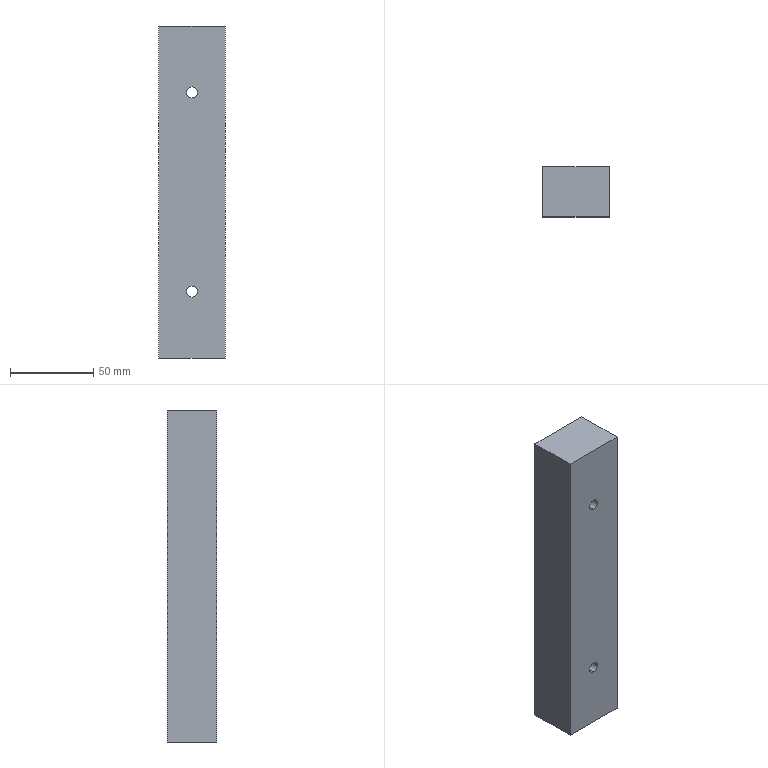Part | SolidWorks | features Extrusion 1, HoleWzd 1 | 1 solid | 16 faces | box 40 x 30 x 200 mm | volume 236731 mm3 | cylinder 8 | plane 8 | commonest cylinder face diameters 6.6 x4 11 x4
STEP:
#1=CARTESIAN_POINT('',(0.,5.,-65.5));
#2=VERTEX_POINT('',#1);
#3=CARTESIAN_POINT('',(0.,5.,-54.5));
#4=VERTEX_POINT('',#3);
#5=CARTESIAN_POINT('',(0.,5.,-60.));
#6=DIRECTION('',(0.,1.,0.));
#7=DIRECTION('',(0.,0.,1.));
#8=AXIS2_PLACEMENT_3D('',#5,#6,#7);
#9=CIRCLE('',#8,5.5);
#10=EDGE_CURVE('',#2,#4,#9,.T.);
#11=ORIENTED_EDGE('',*,*,#10,.F.);
#12=CARTESIAN_POINT('',(0.,15.,-65.5));
#13=VERTEX_POINT('',#12);
#14=CARTESIAN_POINT('',(0.,15.,-65.5));
#15=DIRECTION('',(0.,1.,0.));
#16=VECTOR('',#15,1000.);
#17=LINE('',#14,#16);
#18=EDGE_CURVE('',#2,#13,#17,.T.);
#19=ORIENTED_EDGE('',*,*,#18,.T.);
#20=CARTESIAN_POINT('',(0.,15.,-54.5));
#21=VERTEX_POINT('',#20);
#22=CARTESIAN_POINT('',(0.,15.,-60.));
#23=DIRECTION('',(0.,1.,0.));
#24=DIRECTION('',(0.,0.,1.));
#25=AXIS2_PLACEMENT_3D('',#22,#23,#24);
#26=CIRCLE('',#25,5.5);
#27=EDGE_CURVE('',#13,#21,#26,.T.);
#28=ORIENTED_EDGE('',*,*,#27,.T.);
#29=CARTESIAN_POINT('',(0.,15.,-54.5));
#30=DIRECTION('',(0.,1.,0.));
#31=VECTOR('',#30,1000.);
#32=LINE('',#29,#31);
#33=EDGE_CURVE('',#4,#21,#32,.T.);
#34=ORIENTED_EDGE('',*,*,#33,.F.);
#35=EDGE_LOOP('',(#11,#19,#28,#34));
#36=FACE_OUTER_BOUND('',#35,.T.);
#37=CARTESIAN_POINT('',(0.,15.,-60.));
#38=DIRECTION('',(0.,1.,0.));
#39=DIRECTION('',(0.,0.,1.));
#40=AXIS2_PLACEMENT_3D('',#37,#38,#39);
#41=CYLINDRICAL_SURFACE('',#40,5.5);
#42=ADVANCED_FACE('',(#36),#41,.F.);
#43=CARTESIAN_POINT('',(0.,-15.,-63.3));
#44=VERTEX_POINT('',#43);
#45=CARTESIAN_POINT('',(0.,-15.,-56.7));
#46=VERTEX_POINT('',#45);
#47=CARTESIAN_POINT('',(0.,-15.,-60.));
#48=DIRECTION('',(0.,1.,0.));
#49=DIRECTION('',(0.,0.,1.));
#50=AXIS2_PLACEMENT_3D('',#47,#48,#49);
#51=CIRCLE('',#50,3.3);
#52=EDGE_CURVE('',#44,#46,#51,.T.);
#53=ORIENTED_EDGE('',*,*,#52,.F.);
#54=CARTESIAN_POINT('',(0.,5.,-63.3));
#55=VERTEX_POINT('',#54);
#56=CARTESIAN_POINT('',(0.,15.,-63.3));
#57=DIRECTION('',(0.,1.,0.));
#58=VECTOR('',#57,1000.);
#59=LINE('',#56,#58);
#60=EDGE_CURVE('',#44,#55,#59,.T.);
#61=ORIENTED_EDGE('',*,*,#60,.T.);
#62=CARTESIAN_POINT('',(0.,5.,-56.7));
#63=VERTEX_POINT('',#62);
#64=CARTESIAN_POINT('',(0.,5.,-60.));
#65=DIRECTION('',(0.,1.,0.));
#66=DIRECTION('',(0.,0.,1.));
#67=AXIS2_PLACEMENT_3D('',#64,#65,#66);
#68=CIRCLE('',#67,3.3);
#69=EDGE_CURVE('',#55,#63,#68,.T.);
#70=ORIENTED_EDGE('',*,*,#69,.T.);
#71=CARTESIAN_POINT('',(0.,15.,-56.7));
#72=DIRECTION('',(0.,1.,0.));
#73=VECTOR('',#72,1000.);
#74=LINE('',#71,#73);
#75=EDGE_CURVE('',#46,#63,#74,.T.);
#76=ORIENTED_EDGE('',*,*,#75,.F.);
#77=EDGE_LOOP('',(#53,#61,#70,#76));
#78=FACE_OUTER_BOUND('',#77,.T.);
#79=CARTESIAN_POINT('',(0.,15.,-60.));
#80=DIRECTION('',(0.,1.,0.));
#81=DIRECTION('',(0.,0.,1.));
#82=AXIS2_PLACEMENT_3D('',#79,#80,#81);
#83=CYLINDRICAL_SURFACE('',#82,3.3);
#84=ADVANCED_FACE('',(#78),#83,.F.);
#85=CARTESIAN_POINT('',(0.,5.,54.5));
#86=VERTEX_POINT('',#85);
#87=CARTESIAN_POINT('',(0.,5.,65.5));
#88=VERTEX_POINT('',#87);
#89=CARTESIAN_POINT('',(0.,5.,60.));
#90=DIRECTION('',(0.,1.,0.));
#91=DIRECTION('',(0.,0.,1.));
#92=AXIS2_PLACEMENT_3D('',#89,#90,#91);
#93=CIRCLE('',#92,5.5);
#94=EDGE_CURVE('',#86,#88,#93,.T.);
#95=ORIENTED_EDGE('',*,*,#94,.F.);
#96=CARTESIAN_POINT('',(0.,15.,54.5));
#97=VERTEX_POINT('',#96);
#98=CARTESIAN_POINT('',(0.,15.,54.5));
#99=DIRECTION('',(0.,1.,0.));
#100=VECTOR('',#99,1000.);
#101=LINE('',#98,#100);
#102=EDGE_CURVE('',#86,#97,#101,.T.);
#103=ORIENTED_EDGE('',*,*,#102,.T.);
#104=CARTESIAN_POINT('',(0.,15.,65.5));
#105=VERTEX_POINT('',#104);
#106=CARTESIAN_POINT('',(0.,15.,60.));
#107=DIRECTION('',(0.,1.,0.));
#108=DIRECTION('',(0.,0.,1.));
#109=AXIS2_PLACEMENT_3D('',#106,#107,#108);
#110=CIRCLE('',#109,5.5);
#111=EDGE_CURVE('',#97,#105,#110,.T.);
#112=ORIENTED_EDGE('',*,*,#111,.T.);
#113=CARTESIAN_POINT('',(0.,15.,65.5));
#114=DIRECTION('',(0.,1.,0.));
#115=VECTOR('',#114,1000.);
#116=LINE('',#113,#115);
#117=EDGE_CURVE('',#88,#105,#116,.T.);
#118=ORIENTED_EDGE('',*,*,#117,.F.);
#119=EDGE_LOOP('',(#95,#103,#112,#118));
#120=FACE_OUTER_BOUND('',#119,.T.);
#121=CARTESIAN_POINT('',(0.,15.,60.));
#122=DIRECTION('',(0.,1.,0.));
#123=DIRECTION('',(0.,0.,1.));
#124=AXIS2_PLACEMENT_3D('',#121,#122,#123);
#125=CYLINDRICAL_SURFACE('',#124,5.5);
#126=ADVANCED_FACE('',(#120),#125,.F.);
#127=CARTESIAN_POINT('',(0.,-15.,56.7));
#128=VERTEX_POINT('',#127);
#129=CARTESIAN_POINT('',(0.,-15.,63.3));
#130=VERTEX_POINT('',#129);
#131=CARTESIAN_POINT('',(0.,-15.,60.));
#132=DIRECTION('',(0.,1.,0.));
#133=DIRECTION('',(0.,0.,1.));
#134=AXIS2_PLACEMENT_3D('',#131,#132,#133);
#135=CIRCLE('',#134,3.3);
#136=EDGE_CURVE('',#128,#130,#135,.T.);
#137=ORIENTED_EDGE('',*,*,#136,.F.);
#138=CARTESIAN_POINT('',(0.,5.,56.7));
#139=VERTEX_POINT('',#138);
#140=CARTESIAN_POINT('',(0.,15.,56.7));
#141=DIRECTION('',(0.,1.,0.));
#142=VECTOR('',#141,1000.);
#143=LINE('',#140,#142);
#144=EDGE_CURVE('',#128,#139,#143,.T.);
#145=ORIENTED_EDGE('',*,*,#144,.T.);
#146=CARTESIAN_POINT('',(0.,5.,63.3));
#147=VERTEX_POINT('',#146);
#148=CARTESIAN_POINT('',(0.,5.,60.));
#149=DIRECTION('',(0.,1.,0.));
#150=DIRECTION('',(0.,0.,1.));
#151=AXIS2_PLACEMENT_3D('',#148,#149,#150);
#152=CIRCLE('',#151,3.3);
#153=EDGE_CURVE('',#139,#147,#152,.T.);
#154=ORIENTED_EDGE('',*,*,#153,.T.);
#155=CARTESIAN_POINT('',(0.,15.,63.3));
#156=DIRECTION('',(0.,1.,0.));
#157=VECTOR('',#156,1000.);
#158=LINE('',#155,#157);
#159=EDGE_CURVE('',#130,#147,#158,.T.);
#160=ORIENTED_EDGE('',*,*,#159,.F.);
#161=EDGE_LOOP('',(#137,#145,#154,#160));
#162=FACE_OUTER_BOUND('',#161,.T.);
#163=CARTESIAN_POINT('',(0.,15.,60.));
#164=DIRECTION('',(0.,1.,0.));
#165=DIRECTION('',(0.,0.,1.));
#166=AXIS2_PLACEMENT_3D('',#163,#164,#165);
#167=CYLINDRICAL_SURFACE('',#166,3.3);
#168=ADVANCED_FACE('',(#162),#167,.F.);
#169=CARTESIAN_POINT('',(20.,-15.,100.));
#170=VERTEX_POINT('',#169);
#171=CARTESIAN_POINT('',(20.,-15.,-100.));
#172=VERTEX_POINT('',#171);
#173=CARTESIAN_POINT('',(20.,-15.,100.));
#174=DIRECTION('',(0.,0.,-1.));
#175=VECTOR('',#174,1000.);
#176=LINE('',#173,#175);
#177=EDGE_CURVE('',#170,#172,#176,.T.);
#178=ORIENTED_EDGE('',*,*,#177,.T.);
#179=CARTESIAN_POINT('',(20.,15.,-100.));
#180=VERTEX_POINT('',#179);
#181=CARTESIAN_POINT('',(20.,15.,-100.));
#182=DIRECTION('',(0.,-1.,0.));
#183=VECTOR('',#182,1000.);
#184=LINE('',#181,#183);
#185=EDGE_CURVE('',#180,#172,#184,.T.);
#186=ORIENTED_EDGE('',*,*,#185,.F.);
#187=CARTESIAN_POINT('',(20.,15.,100.));
#188=VERTEX_POINT('',#187);
#189=CARTESIAN_POINT('',(20.,15.,100.));
#190=DIRECTION('',(0.,0.,-1.));
#191=VECTOR('',#190,1000.);
#192=LINE('',#189,#191);
#193=EDGE_CURVE('',#188,#180,#192,.T.);
#194=ORIENTED_EDGE('',*,*,#193,.F.);
#195=CARTESIAN_POINT('',(20.,15.,100.));
#196=DIRECTION('',(0.,-1.,0.));
#197=VECTOR('',#196,1000.);
#198=LINE('',#195,#197);
#199=EDGE_CURVE('',#188,#170,#198,.T.);
#200=ORIENTED_EDGE('',*,*,#199,.T.);
#201=EDGE_LOOP('',(#178,#186,#194,#200));
#202=FACE_OUTER_BOUND('',#201,.T.);
#203=CARTESIAN_POINT('',(20.,15.,100.));
#204=DIRECTION('',(-1.,0.,0.));
#205=DIRECTION('',(0.,0.,1.));
#206=AXIS2_PLACEMENT_3D('',#203,#204,#205);
#207=PLANE('',#206);
#208=ADVANCED_FACE('',(#202),#207,.F.);
#209=CARTESIAN_POINT('',(-20.,-15.,-100.));
#210=VERTEX_POINT('',#209);
#211=CARTESIAN_POINT('',(-20.,-15.,-100.));
#212=DIRECTION('',(-1.,0.,0.));
#213=VECTOR('',#212,1000.);
#214=LINE('',#211,#213);
#215=EDGE_CURVE('',#172,#210,#214,.T.);
#216=ORIENTED_EDGE('',*,*,#215,.T.);
#217=CARTESIAN_POINT('',(-20.,15.,-100.));
#218=VERTEX_POINT('',#217);
#219=CARTESIAN_POINT('',(-20.,15.,-100.));
#220=DIRECTION('',(0.,-1.,0.));
#221=VECTOR('',#220,1000.);
#222=LINE('',#219,#221);
#223=EDGE_CURVE('',#218,#210,#222,.T.);
#224=ORIENTED_EDGE('',*,*,#223,.F.);
#225=CARTESIAN_POINT('',(-20.,15.,-100.));
#226=DIRECTION('',(-1.,0.,0.));
#227=VECTOR('',#226,1000.);
#228=LINE('',#225,#227);
#229=EDGE_CURVE('',#180,#218,#228,.T.);
#230=ORIENTED_EDGE('',*,*,#229,.F.);
#231=ORIENTED_EDGE('',*,*,#185,.T.);
#232=EDGE_LOOP('',(#216,#224,#230,#231));
#233=FACE_OUTER_BOUND('',#232,.T.);
#234=CARTESIAN_POINT('',(-20.,15.,-100.));
#235=DIRECTION('',(0.,0.,1.));
#236=DIRECTION('',(1.,0.,0.));
#237=AXIS2_PLACEMENT_3D('',#234,#235,#236);
#238=PLANE('',#237);
#239=ADVANCED_FACE('',(#233),#238,.F.);
#240=CARTESIAN_POINT('',(-20.,-15.,100.));
#241=VERTEX_POINT('',#240);
#242=CARTESIAN_POINT('',(-20.,-15.,100.));
#243=DIRECTION('',(0.,0.,1.));
#244=VECTOR('',#243,1000.);
#245=LINE('',#242,#244);
#246=EDGE_CURVE('',#210,#241,#245,.T.);
#247=ORIENTED_EDGE('',*,*,#246,.T.);
#248=CARTESIAN_POINT('',(-20.,15.,100.));
#249=VERTEX_POINT('',#248);
#250=CARTESIAN_POINT('',(-20.,15.,100.));
#251=DIRECTION('',(0.,-1.,0.));
#252=VECTOR('',#251,1000.);
#253=LINE('',#250,#252);
#254=EDGE_CURVE('',#249,#241,#253,.T.);
#255=ORIENTED_EDGE('',*,*,#254,.F.);
#256=CARTESIAN_POINT('',(-20.,15.,100.));
#257=DIRECTION('',(0.,0.,1.));
#258=VECTOR('',#257,1000.);
#259=LINE('',#256,#258);
#260=EDGE_CURVE('',#218,#249,#259,.T.);
#261=ORIENTED_EDGE('',*,*,#260,.F.);
#262=ORIENTED_EDGE('',*,*,#223,.T.);
#263=EDGE_LOOP('',(#247,#255,#261,#262));
#264=FACE_OUTER_BOUND('',#263,.T.);
#265=CARTESIAN_POINT('',(-20.,15.,100.));
#266=DIRECTION('',(1.,0.,0.));
#267=DIRECTION('',(0.,0.,-1.));
#268=AXIS2_PLACEMENT_3D('',#265,#266,#267);
#269=PLANE('',#268);
#270=ADVANCED_FACE('',(#264),#269,.F.);
#271=CARTESIAN_POINT('',(-20.,-15.,100.));
#272=DIRECTION('',(1.,0.,0.));
#273=VECTOR('',#272,1000.);
#274=LINE('',#271,#273);
#275=EDGE_CURVE('',#241,#170,#274,.T.);
#276=ORIENTED_EDGE('',*,*,#275,.T.);
#277=ORIENTED_EDGE('',*,*,#199,.F.);
#278=CARTESIAN_POINT('',(-20.,15.,100.));
#279=DIRECTION('',(1.,0.,0.));
#280=VECTOR('',#279,1000.);
#281=LINE('',#278,#280);
#282=EDGE_CURVE('',#249,#188,#281,.T.);
#283=ORIENTED_EDGE('',*,*,#282,.F.);
#284=ORIENTED_EDGE('',*,*,#254,.T.);
#285=EDGE_LOOP('',(#276,#277,#283,#284));
#286=FACE_OUTER_BOUND('',#285,.T.);
#287=CARTESIAN_POINT('',(-20.,15.,100.));
#288=DIRECTION('',(0.,0.,-1.));
#289=DIRECTION('',(-1.,0.,0.));
#290=AXIS2_PLACEMENT_3D('',#287,#288,#289);
#291=PLANE('',#290);
#292=ADVANCED_FACE('',(#286),#291,.F.);
#293=CARTESIAN_POINT('',(0.,15.,-60.));
#294=DIRECTION('',(0.,1.,0.));
#295=DIRECTION('',(0.,0.,1.));
#296=AXIS2_PLACEMENT_3D('',#293,#294,#295);
#297=CIRCLE('',#296,5.5);
#298=EDGE_CURVE('',#21,#13,#297,.T.);
#299=ORIENTED_EDGE('',*,*,#298,.F.);
#300=ORIENTED_EDGE('',*,*,#27,.F.);
#301=EDGE_LOOP('',(#299,#300));
#302=FACE_BOUND('',#301,.T.);
#303=CARTESIAN_POINT('',(0.,15.,60.));
#304=DIRECTION('',(0.,1.,0.));
#305=DIRECTION('',(0.,0.,1.));
#306=AXIS2_PLACEMENT_3D('',#303,#304,#305);
#307=CIRCLE('',#306,5.5);
#308=EDGE_CURVE('',#105,#97,#307,.T.);
#309=ORIENTED_EDGE('',*,*,#308,.F.);
#310=ORIENTED_EDGE('',*,*,#111,.F.);
#311=EDGE_LOOP('',(#309,#310));
#312=FACE_BOUND('',#311,.T.);
#313=ORIENTED_EDGE('',*,*,#193,.T.);
#314=ORIENTED_EDGE('',*,*,#229,.T.);
#315=ORIENTED_EDGE('',*,*,#260,.T.);
#316=ORIENTED_EDGE('',*,*,#282,.T.);
#317=EDGE_LOOP('',(#313,#314,#315,#316));
#318=FACE_OUTER_BOUND('',#317,.T.);
#319=CARTESIAN_POINT('',(0.,15.,0.));
#320=DIRECTION('',(0.,-1.,0.));
#321=DIRECTION('',(0.,0.,-1.));
#322=AXIS2_PLACEMENT_3D('',#319,#320,#321);
#323=PLANE('',#322);
#324=ADVANCED_FACE('',(#302,#312,#318),#323,.F.);
#325=CARTESIAN_POINT('',(0.,-15.,-60.));
#326=DIRECTION('',(0.,1.,0.));
#327=DIRECTION('',(0.,0.,1.));
#328=AXIS2_PLACEMENT_3D('',#325,#326,#327);
#329=CIRCLE('',#328,3.3);
#330=EDGE_CURVE('',#46,#44,#329,.T.);
#331=ORIENTED_EDGE('',*,*,#330,.T.);
#332=ORIENTED_EDGE('',*,*,#52,.T.);
#333=EDGE_LOOP('',(#331,#332));
#334=FACE_BOUND('',#333,.T.);
#335=CARTESIAN_POINT('',(0.,-15.,60.));
#336=DIRECTION('',(0.,1.,0.));
#337=DIRECTION('',(0.,0.,1.));
#338=AXIS2_PLACEMENT_3D('',#335,#336,#337);
#339=CIRCLE('',#338,3.3);
#340=EDGE_CURVE('',#130,#128,#339,.T.);
#341=ORIENTED_EDGE('',*,*,#340,.T.);
#342=ORIENTED_EDGE('',*,*,#136,.T.);
#343=EDGE_LOOP('',(#341,#342));
#344=FACE_BOUND('',#343,.T.);
#345=ORIENTED_EDGE('',*,*,#177,.F.);
#346=ORIENTED_EDGE('',*,*,#275,.F.);
#347=ORIENTED_EDGE('',*,*,#246,.F.);
#348=ORIENTED_EDGE('',*,*,#215,.F.);
#349=EDGE_LOOP('',(#345,#346,#347,#348));
#350=FACE_OUTER_BOUND('',#349,.T.);
#351=CARTESIAN_POINT('',(0.,-15.,0.));
#352=DIRECTION('',(0.,-1.,0.));
#353=DIRECTION('',(0.,0.,-1.));
#354=AXIS2_PLACEMENT_3D('',#351,#352,#353);
#355=PLANE('',#354);
#356=ADVANCED_FACE('',(#334,#344,#350),#355,.T.);
#357=ORIENTED_EDGE('',*,*,#144,.F.);
#358=ORIENTED_EDGE('',*,*,#340,.F.);
#359=ORIENTED_EDGE('',*,*,#159,.T.);
#360=CARTESIAN_POINT('',(0.,5.,60.));
#361=DIRECTION('',(0.,1.,0.));
#362=DIRECTION('',(0.,0.,1.));
#363=AXIS2_PLACEMENT_3D('',#360,#361,#362);
#364=CIRCLE('',#363,3.3);
#365=EDGE_CURVE('',#147,#139,#364,.T.);
#366=ORIENTED_EDGE('',*,*,#365,.T.);
#367=EDGE_LOOP('',(#357,#358,#359,#366));
#368=FACE_OUTER_BOUND('',#367,.T.);
#369=CARTESIAN_POINT('',(0.,15.,60.));
#370=DIRECTION('',(0.,1.,0.));
#371=DIRECTION('',(0.,0.,1.));
#372=AXIS2_PLACEMENT_3D('',#369,#370,#371);
#373=CYLINDRICAL_SURFACE('',#372,3.3);
#374=ADVANCED_FACE('',(#368),#373,.F.);
#375=ORIENTED_EDGE('',*,*,#365,.F.);
#376=ORIENTED_EDGE('',*,*,#153,.F.);
#377=EDGE_LOOP('',(#375,#376));
#378=FACE_BOUND('',#377,.T.);
#379=CARTESIAN_POINT('',(0.,5.,60.));
#380=DIRECTION('',(0.,1.,0.));
#381=DIRECTION('',(0.,0.,1.));
#382=AXIS2_PLACEMENT_3D('',#379,#380,#381);
#383=CIRCLE('',#382,5.5);
#384=EDGE_CURVE('',#88,#86,#383,.T.);
#385=ORIENTED_EDGE('',*,*,#384,.T.);
#386=ORIENTED_EDGE('',*,*,#94,.T.);
#387=EDGE_LOOP('',(#385,#386));
#388=FACE_OUTER_BOUND('',#387,.T.);
#389=CARTESIAN_POINT('',(3.3,5.,60.));
#390=DIRECTION('',(0.,-1.,0.));
#391=DIRECTION('',(0.,0.,-1.));
#392=AXIS2_PLACEMENT_3D('',#389,#390,#391);
#393=PLANE('',#392);
#394=ADVANCED_FACE('',(#378,#388),#393,.F.);
#395=ORIENTED_EDGE('',*,*,#102,.F.);
#396=ORIENTED_EDGE('',*,*,#384,.F.);
#397=ORIENTED_EDGE('',*,*,#117,.T.);
#398=ORIENTED_EDGE('',*,*,#308,.T.);
#399=EDGE_LOOP('',(#395,#396,#397,#398));
#400=FACE_OUTER_BOUND('',#399,.T.);
#401=CARTESIAN_POINT('',(0.,15.,60.));
#402=DIRECTION('',(0.,1.,0.));
#403=DIRECTION('',(0.,0.,1.));
#404=AXIS2_PLACEMENT_3D('',#401,#402,#403);
#405=CYLINDRICAL_SURFACE('',#404,5.5);
#406=ADVANCED_FACE('',(#400),#405,.F.);
#407=ORIENTED_EDGE('',*,*,#60,.F.);
#408=ORIENTED_EDGE('',*,*,#330,.F.);
#409=ORIENTED_EDGE('',*,*,#75,.T.);
#410=CARTESIAN_POINT('',(0.,5.,-60.));
#411=DIRECTION('',(0.,1.,0.));
#412=DIRECTION('',(0.,0.,1.));
#413=AXIS2_PLACEMENT_3D('',#410,#411,#412);
#414=CIRCLE('',#413,3.3);
#415=EDGE_CURVE('',#63,#55,#414,.T.);
#416=ORIENTED_EDGE('',*,*,#415,.T.);
#417=EDGE_LOOP('',(#407,#408,#409,#416));
#418=FACE_OUTER_BOUND('',#417,.T.);
#419=CARTESIAN_POINT('',(0.,15.,-60.));
#420=DIRECTION('',(0.,1.,0.));
#421=DIRECTION('',(0.,0.,1.));
#422=AXIS2_PLACEMENT_3D('',#419,#420,#421);
#423=CYLINDRICAL_SURFACE('',#422,3.3);
#424=ADVANCED_FACE('',(#418),#423,.F.);
#425=ORIENTED_EDGE('',*,*,#415,.F.);
#426=ORIENTED_EDGE('',*,*,#69,.F.);
#427=EDGE_LOOP('',(#425,#426));
#428=FACE_BOUND('',#427,.T.);
#429=CARTESIAN_POINT('',(0.,5.,-60.));
#430=DIRECTION('',(0.,1.,0.));
#431=DIRECTION('',(0.,0.,1.));
#432=AXIS2_PLACEMENT_3D('',#429,#430,#431);
#433=CIRCLE('',#432,5.5);
#434=EDGE_CURVE('',#4,#2,#433,.T.);
#435=ORIENTED_EDGE('',*,*,#434,.T.);
#436=ORIENTED_EDGE('',*,*,#10,.T.);
#437=EDGE_LOOP('',(#435,#436));
#438=FACE_OUTER_BOUND('',#437,.T.);
#439=CARTESIAN_POINT('',(3.3,5.,-60.));
#440=DIRECTION('',(0.,-1.,0.));
#441=DIRECTION('',(0.,0.,-1.));
#442=AXIS2_PLACEMENT_3D('',#439,#440,#441);
#443=PLANE('',#442);
#444=ADVANCED_FACE('',(#428,#438),#443,.F.);
#445=ORIENTED_EDGE('',*,*,#18,.F.);
#446=ORIENTED_EDGE('',*,*,#434,.F.);
#447=ORIENTED_EDGE('',*,*,#33,.T.);
#448=ORIENTED_EDGE('',*,*,#298,.T.);
#449=EDGE_LOOP('',(#445,#446,#447,#448));
#450=FACE_OUTER_BOUND('',#449,.T.);
#451=CARTESIAN_POINT('',(0.,15.,-60.));
#452=DIRECTION('',(0.,1.,0.));
#453=DIRECTION('',(0.,0.,1.));
#454=AXIS2_PLACEMENT_3D('',#451,#452,#453);
#455=CYLINDRICAL_SURFACE('',#454,5.5);
#456=ADVANCED_FACE('',(#450),#455,.F.);
#457=CLOSED_SHELL('',(#42,#84,#126,#168,#208,#239,#270,#292,#324,#356,#374,#394,#406,#424,#444,#456));
#458=MANIFOLD_SOLID_BREP('',#457);
#459=CARTESIAN_POINT('',(0.,0.,0.));
#460=DIRECTION('',(0.,0.,1.));
#461=DIRECTION('',(1.,0.,0.));
#462=AXIS2_PLACEMENT_3D('',#459,#460,#461);
#463=(LENGTH_UNIT()NAMED_UNIT(*)SI_UNIT(.MILLI.,.METRE.));
#464=UNCERTAINTY_MEASURE_WITH_UNIT(LENGTH_MEASURE(0.00001),#463,'','');
#465=(NAMED_UNIT(*)PLANE_ANGLE_UNIT()SI_UNIT($,.RADIAN.));
#466=(NAMED_UNIT(*)SI_UNIT($,.STERADIAN.)SOLID_ANGLE_UNIT());
#467=(GEOMETRIC_REPRESENTATION_CONTEXT(3)GLOBAL_UNCERTAINTY_ASSIGNED_CONTEXT((#464))GLOBAL_UNIT_ASSIGNED_CONTEXT((#463,#465,#466))REPRESENTATION_CONTEXT('',''));
#468=ADVANCED_BREP_SHAPE_REPRESENTATION('',(#458,#462),#467);